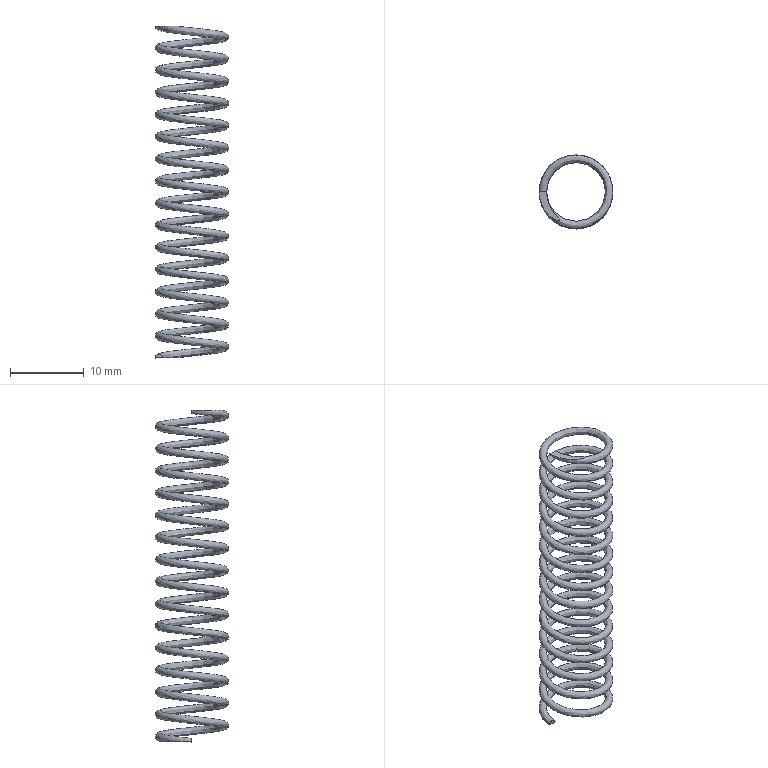Part | STEP file | gslz 2016.10.28-6_id374_x_t | 1 solid | 5 faces | box 9.997 x 9.994 x 45 mm | volume 330.149 mm3 | plane 4 | spline 1